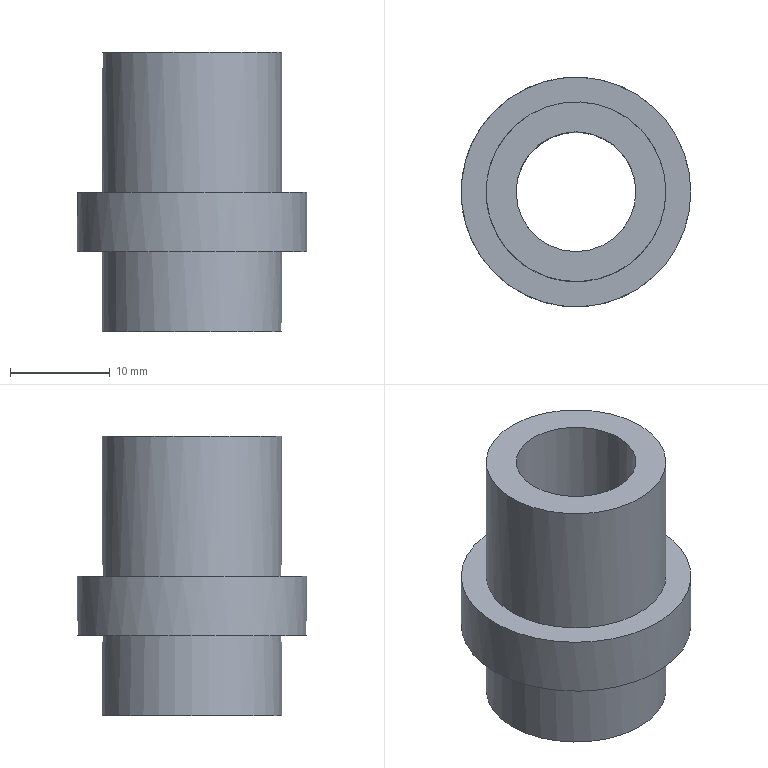Part | STEP file | solid 37 | 1 solid | 8 faces | box 23 x 23 x 28 mm | volume 4924 mm3 | cylinder 4 | plane 4 | commonest cylinder face diameters 18 x2 12 x1 23 x1